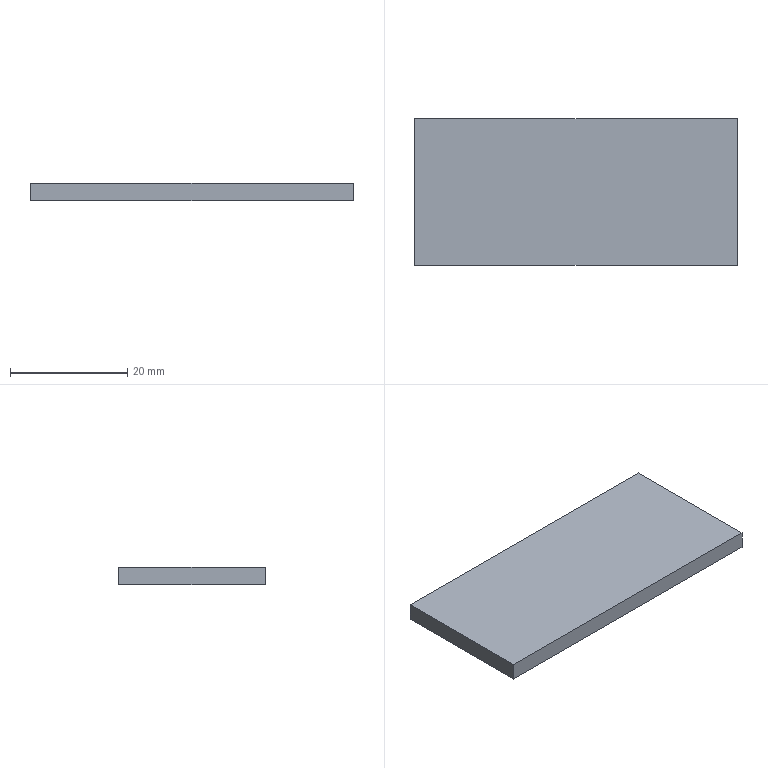Part | STEP file | 7101204 | 1 solid | 6 faces | box 55 x 25 x 3 mm | volume 4125 mm3 | plane 6
STEP:
#1=CARTESIAN_POINT('',(0.,0.,0.));
#2=DIRECTION('',(0.,0.,1.));
#3=DIRECTION('',(1.,0.,0.));
#4=AXIS2_PLACEMENT_3D('',#1,#2,#3);
#5=CARTESIAN_POINT('',(-56.43,-3.671,0.));
#6=VERTEX_POINT('',#5);
#7=CARTESIAN_POINT('',(-56.43,-28.671,0.));
#8=VERTEX_POINT('',#7);
#9=CARTESIAN_POINT('',(-56.43,-3.671,0.));
#10=DIRECTION('',(0.,-1.,0.));
#11=VECTOR('',#10,1.);
#12=LINE('',#9,#11);
#13=CARTESIAN_POINT('',(-56.43,-3.671,3.));
#14=DIRECTION('',(1.,0.,0.));
#15=DIRECTION('',(0.,1.,0.));
#16=AXIS2_PLACEMENT_3D('',#13,#14,#15);
#17=PLANE('',#16);
#18=CARTESIAN_POINT('',(0.,-3.));
#19=DIRECTION('',(-1.,0.));
#20=VECTOR('',#19,1.);
#21=LINE('',#18,#20);
#22=(GEOMETRIC_REPRESENTATION_CONTEXT(2)PARAMETRIC_REPRESENTATION_CONTEXT()REPRESENTATION_CONTEXT('',''));
#23=DEFINITIONAL_REPRESENTATION('',(#21),#22);
#24=PCURVE('',#17,#23);
#25=CARTESIAN_POINT('',(-56.43,-28.671,0.));
#26=DIRECTION('',(0.,0.,1.));
#27=DIRECTION('',(1.,0.,0.));
#28=AXIS2_PLACEMENT_3D('',#25,#26,#27);
#29=PLANE('',#28);
#30=CARTESIAN_POINT('',(0.,25.));
#31=DIRECTION('',(0.,-1.));
#32=VECTOR('',#31,1.);
#33=LINE('',#30,#32);
#34=(GEOMETRIC_REPRESENTATION_CONTEXT(2)PARAMETRIC_REPRESENTATION_CONTEXT()REPRESENTATION_CONTEXT('',''));
#35=DEFINITIONAL_REPRESENTATION('',(#33),#34);
#36=PCURVE('',#29,#35);
#37=SURFACE_CURVE('',#12,(#24,#36),.PCURVE_S1.);
#38=EDGE_CURVE('',#6,#8,#37,.T.);
#39=ORIENTED_EDGE('',*,*,#38,.T.);
#40=CARTESIAN_POINT('',(-56.43,-28.671,3.));
#41=VERTEX_POINT('',#40);
#42=CARTESIAN_POINT('',(-56.43,-28.671,3.));
#43=DIRECTION('',(0.,0.,-1.));
#44=VECTOR('',#43,1.);
#45=LINE('',#42,#44);
#46=CARTESIAN_POINT('',(-25.,0.));
#47=DIRECTION('',(0.,-1.));
#48=VECTOR('',#47,1.);
#49=LINE('',#46,#48);
#50=(GEOMETRIC_REPRESENTATION_CONTEXT(2)PARAMETRIC_REPRESENTATION_CONTEXT()REPRESENTATION_CONTEXT('',''));
#51=DEFINITIONAL_REPRESENTATION('',(#49),#50);
#52=PCURVE('',#17,#51);
#53=CARTESIAN_POINT('',(-56.43,-28.671,3.));
#54=DIRECTION('',(0.,1.,0.));
#55=DIRECTION('',(0.,0.,1.));
#56=AXIS2_PLACEMENT_3D('',#53,#54,#55);
#57=PLANE('',#56);
#58=CARTESIAN_POINT('',(0.,0.));
#59=DIRECTION('',(-1.,0.));
#60=VECTOR('',#59,1.);
#61=LINE('',#58,#60);
#62=(GEOMETRIC_REPRESENTATION_CONTEXT(2)PARAMETRIC_REPRESENTATION_CONTEXT()REPRESENTATION_CONTEXT('',''));
#63=DEFINITIONAL_REPRESENTATION('',(#61),#62);
#64=PCURVE('',#57,#63);
#65=SURFACE_CURVE('',#45,(#52,#64),.PCURVE_S1.);
#66=EDGE_CURVE('',#41,#8,#65,.T.);
#67=ORIENTED_EDGE('',*,*,#66,.F.);
#68=CARTESIAN_POINT('',(-56.43,-3.671,3.));
#69=VERTEX_POINT('',#68);
#70=CARTESIAN_POINT('',(-56.43,-3.671,3.));
#71=DIRECTION('',(0.,-1.,0.));
#72=VECTOR('',#71,1.);
#73=LINE('',#70,#72);
#74=CARTESIAN_POINT('',(0.,0.));
#75=DIRECTION('',(-1.,0.));
#76=VECTOR('',#75,1.);
#77=LINE('',#74,#76);
#78=(GEOMETRIC_REPRESENTATION_CONTEXT(2)PARAMETRIC_REPRESENTATION_CONTEXT()REPRESENTATION_CONTEXT('',''));
#79=DEFINITIONAL_REPRESENTATION('',(#77),#78);
#80=PCURVE('',#17,#79);
#81=CARTESIAN_POINT('',(-56.43,-28.671,3.));
#82=DIRECTION('',(0.,0.,1.));
#83=DIRECTION('',(1.,0.,0.));
#84=AXIS2_PLACEMENT_3D('',#81,#82,#83);
#85=PLANE('',#84);
#86=CARTESIAN_POINT('',(0.,25.));
#87=DIRECTION('',(0.,-1.));
#88=VECTOR('',#87,1.);
#89=LINE('',#86,#88);
#90=(GEOMETRIC_REPRESENTATION_CONTEXT(2)PARAMETRIC_REPRESENTATION_CONTEXT()REPRESENTATION_CONTEXT('',''));
#91=DEFINITIONAL_REPRESENTATION('',(#89),#90);
#92=PCURVE('',#85,#91);
#93=SURFACE_CURVE('',#73,(#80,#92),.PCURVE_S1.);
#94=EDGE_CURVE('',#69,#41,#93,.T.);
#95=ORIENTED_EDGE('',*,*,#94,.F.);
#96=CARTESIAN_POINT('',(-56.43,-3.671,3.));
#97=DIRECTION('',(0.,0.,-1.));
#98=VECTOR('',#97,1.);
#99=LINE('',#96,#98);
#100=CARTESIAN_POINT('',(0.,0.));
#101=DIRECTION('',(0.,-1.));
#102=VECTOR('',#101,1.);
#103=LINE('',#100,#102);
#104=(GEOMETRIC_REPRESENTATION_CONTEXT(2)PARAMETRIC_REPRESENTATION_CONTEXT()REPRESENTATION_CONTEXT('',''));
#105=DEFINITIONAL_REPRESENTATION('',(#103),#104);
#106=PCURVE('',#17,#105);
#107=CARTESIAN_POINT('',(-56.43,-3.671,3.));
#108=DIRECTION('',(0.,-1.,0.));
#109=DIRECTION('',(0.,0.,-1.));
#110=AXIS2_PLACEMENT_3D('',#107,#108,#109);
#111=PLANE('',#110);
#112=CARTESIAN_POINT('',(0.,0.));
#113=DIRECTION('',(1.,0.));
#114=VECTOR('',#113,1.);
#115=LINE('',#112,#114);
#116=(GEOMETRIC_REPRESENTATION_CONTEXT(2)PARAMETRIC_REPRESENTATION_CONTEXT()REPRESENTATION_CONTEXT('',''));
#117=DEFINITIONAL_REPRESENTATION('',(#115),#116);
#118=PCURVE('',#111,#117);
#119=SURFACE_CURVE('',#99,(#106,#118),.PCURVE_S1.);
#120=EDGE_CURVE('',#69,#6,#119,.T.);
#121=ORIENTED_EDGE('',*,*,#120,.T.);
#122=EDGE_LOOP('',(#39,#67,#95,#121));
#123=FACE_BOUND('',#122,.T.);
#124=ADVANCED_FACE('',(#123),#17,.F.);
#125=CARTESIAN_POINT('',(-1.43,-28.671,0.));
#126=VERTEX_POINT('',#125);
#127=CARTESIAN_POINT('',(-56.43,-28.671,0.));
#128=DIRECTION('',(1.,0.,0.));
#129=VECTOR('',#128,1.);
#130=LINE('',#127,#129);
#131=CARTESIAN_POINT('',(-3.,0.));
#132=DIRECTION('',(0.,1.));
#133=VECTOR('',#132,1.);
#134=LINE('',#131,#133);
#135=(GEOMETRIC_REPRESENTATION_CONTEXT(2)PARAMETRIC_REPRESENTATION_CONTEXT()REPRESENTATION_CONTEXT('',''));
#136=DEFINITIONAL_REPRESENTATION('',(#134),#135);
#137=PCURVE('',#57,#136);
#138=CARTESIAN_POINT('',(0.,0.));
#139=DIRECTION('',(1.,0.));
#140=VECTOR('',#139,1.);
#141=LINE('',#138,#140);
#142=(GEOMETRIC_REPRESENTATION_CONTEXT(2)PARAMETRIC_REPRESENTATION_CONTEXT()REPRESENTATION_CONTEXT('',''));
#143=DEFINITIONAL_REPRESENTATION('',(#141),#142);
#144=PCURVE('',#29,#143);
#145=SURFACE_CURVE('',#130,(#137,#144),.PCURVE_S1.);
#146=EDGE_CURVE('',#8,#126,#145,.T.);
#147=ORIENTED_EDGE('',*,*,#146,.T.);
#148=CARTESIAN_POINT('',(-1.43,-28.671,3.));
#149=VERTEX_POINT('',#148);
#150=CARTESIAN_POINT('',(-1.43,-28.671,3.));
#151=DIRECTION('',(0.,0.,-1.));
#152=VECTOR('',#151,1.);
#153=LINE('',#150,#152);
#154=CARTESIAN_POINT('',(0.,55.));
#155=DIRECTION('',(-1.,0.));
#156=VECTOR('',#155,1.);
#157=LINE('',#154,#156);
#158=(GEOMETRIC_REPRESENTATION_CONTEXT(2)PARAMETRIC_REPRESENTATION_CONTEXT()REPRESENTATION_CONTEXT('',''));
#159=DEFINITIONAL_REPRESENTATION('',(#157),#158);
#160=PCURVE('',#57,#159);
#161=CARTESIAN_POINT('',(-1.43,-3.671,3.));
#162=DIRECTION('',(-1.,0.,0.));
#163=DIRECTION('',(0.,0.,1.));
#164=AXIS2_PLACEMENT_3D('',#161,#162,#163);
#165=PLANE('',#164);
#166=CARTESIAN_POINT('',(0.,-25.));
#167=DIRECTION('',(-1.,0.));
#168=VECTOR('',#167,1.);
#169=LINE('',#166,#168);
#170=(GEOMETRIC_REPRESENTATION_CONTEXT(2)PARAMETRIC_REPRESENTATION_CONTEXT()REPRESENTATION_CONTEXT('',''));
#171=DEFINITIONAL_REPRESENTATION('',(#169),#170);
#172=PCURVE('',#165,#171);
#173=SURFACE_CURVE('',#153,(#160,#172),.PCURVE_S1.);
#174=EDGE_CURVE('',#149,#126,#173,.T.);
#175=ORIENTED_EDGE('',*,*,#174,.F.);
#176=CARTESIAN_POINT('',(-56.43,-28.671,3.));
#177=DIRECTION('',(1.,0.,0.));
#178=VECTOR('',#177,1.);
#179=LINE('',#176,#178);
#180=CARTESIAN_POINT('',(0.,0.));
#181=DIRECTION('',(0.,1.));
#182=VECTOR('',#181,1.);
#183=LINE('',#180,#182);
#184=(GEOMETRIC_REPRESENTATION_CONTEXT(2)PARAMETRIC_REPRESENTATION_CONTEXT()REPRESENTATION_CONTEXT('',''));
#185=DEFINITIONAL_REPRESENTATION('',(#183),#184);
#186=PCURVE('',#57,#185);
#187=CARTESIAN_POINT('',(0.,0.));
#188=DIRECTION('',(1.,0.));
#189=VECTOR('',#188,1.);
#190=LINE('',#187,#189);
#191=(GEOMETRIC_REPRESENTATION_CONTEXT(2)PARAMETRIC_REPRESENTATION_CONTEXT()REPRESENTATION_CONTEXT('',''));
#192=DEFINITIONAL_REPRESENTATION('',(#190),#191);
#193=PCURVE('',#85,#192);
#194=SURFACE_CURVE('',#179,(#186,#193),.PCURVE_S1.);
#195=EDGE_CURVE('',#41,#149,#194,.T.);
#196=ORIENTED_EDGE('',*,*,#195,.F.);
#197=ORIENTED_EDGE('',*,*,#66,.T.);
#198=EDGE_LOOP('',(#147,#175,#196,#197));
#199=FACE_BOUND('',#198,.T.);
#200=ADVANCED_FACE('',(#199),#57,.F.);
#201=CARTESIAN_POINT('',(-1.43,-3.671,0.));
#202=VERTEX_POINT('',#201);
#203=CARTESIAN_POINT('',(-1.43,-3.671,0.));
#204=DIRECTION('',(0.,1.,0.));
#205=VECTOR('',#204,1.);
#206=LINE('',#203,#205);
#207=CARTESIAN_POINT('',(-3.,0.));
#208=DIRECTION('',(0.,1.));
#209=VECTOR('',#208,1.);
#210=LINE('',#207,#209);
#211=(GEOMETRIC_REPRESENTATION_CONTEXT(2)PARAMETRIC_REPRESENTATION_CONTEXT()REPRESENTATION_CONTEXT('',''));
#212=DEFINITIONAL_REPRESENTATION('',(#210),#211);
#213=PCURVE('',#165,#212);
#214=CARTESIAN_POINT('',(55.,25.));
#215=DIRECTION('',(0.,1.));
#216=VECTOR('',#215,1.);
#217=LINE('',#214,#216);
#218=(GEOMETRIC_REPRESENTATION_CONTEXT(2)PARAMETRIC_REPRESENTATION_CONTEXT()REPRESENTATION_CONTEXT('',''));
#219=DEFINITIONAL_REPRESENTATION('',(#217),#218);
#220=PCURVE('',#29,#219);
#221=SURFACE_CURVE('',#206,(#213,#220),.PCURVE_S1.);
#222=EDGE_CURVE('',#126,#202,#221,.T.);
#223=ORIENTED_EDGE('',*,*,#222,.T.);
#224=CARTESIAN_POINT('',(-1.43,-3.671,3.));
#225=VERTEX_POINT('',#224);
#226=CARTESIAN_POINT('',(-1.43,-3.671,3.));
#227=DIRECTION('',(0.,0.,-1.));
#228=VECTOR('',#227,1.);
#229=LINE('',#226,#228);
#230=CARTESIAN_POINT('',(0.,0.));
#231=DIRECTION('',(-1.,0.));
#232=VECTOR('',#231,1.);
#233=LINE('',#230,#232);
#234=(GEOMETRIC_REPRESENTATION_CONTEXT(2)PARAMETRIC_REPRESENTATION_CONTEXT()REPRESENTATION_CONTEXT('',''));
#235=DEFINITIONAL_REPRESENTATION('',(#233),#234);
#236=PCURVE('',#165,#235);
#237=CARTESIAN_POINT('',(0.,55.));
#238=DIRECTION('',(1.,0.));
#239=VECTOR('',#238,1.);
#240=LINE('',#237,#239);
#241=(GEOMETRIC_REPRESENTATION_CONTEXT(2)PARAMETRIC_REPRESENTATION_CONTEXT()REPRESENTATION_CONTEXT('',''));
#242=DEFINITIONAL_REPRESENTATION('',(#240),#241);
#243=PCURVE('',#111,#242);
#244=SURFACE_CURVE('',#229,(#236,#243),.PCURVE_S1.);
#245=EDGE_CURVE('',#225,#202,#244,.T.);
#246=ORIENTED_EDGE('',*,*,#245,.F.);
#247=CARTESIAN_POINT('',(-1.43,-3.671,3.));
#248=DIRECTION('',(0.,1.,0.));
#249=VECTOR('',#248,1.);
#250=LINE('',#247,#249);
#251=CARTESIAN_POINT('',(0.,0.));
#252=DIRECTION('',(0.,1.));
#253=VECTOR('',#252,1.);
#254=LINE('',#251,#253);
#255=(GEOMETRIC_REPRESENTATION_CONTEXT(2)PARAMETRIC_REPRESENTATION_CONTEXT()REPRESENTATION_CONTEXT('',''));
#256=DEFINITIONAL_REPRESENTATION('',(#254),#255);
#257=PCURVE('',#165,#256);
#258=CARTESIAN_POINT('',(55.,25.));
#259=DIRECTION('',(0.,1.));
#260=VECTOR('',#259,1.);
#261=LINE('',#258,#260);
#262=(GEOMETRIC_REPRESENTATION_CONTEXT(2)PARAMETRIC_REPRESENTATION_CONTEXT()REPRESENTATION_CONTEXT('',''));
#263=DEFINITIONAL_REPRESENTATION('',(#261),#262);
#264=PCURVE('',#85,#263);
#265=SURFACE_CURVE('',#250,(#257,#264),.PCURVE_S1.);
#266=EDGE_CURVE('',#149,#225,#265,.T.);
#267=ORIENTED_EDGE('',*,*,#266,.F.);
#268=ORIENTED_EDGE('',*,*,#174,.T.);
#269=EDGE_LOOP('',(#223,#246,#267,#268));
#270=FACE_BOUND('',#269,.T.);
#271=ADVANCED_FACE('',(#270),#165,.F.);
#272=CARTESIAN_POINT('',(-56.43,-3.671,0.));
#273=DIRECTION('',(-1.,0.,0.));
#274=VECTOR('',#273,1.);
#275=LINE('',#272,#274);
#276=CARTESIAN_POINT('',(3.,0.));
#277=DIRECTION('',(0.,-1.));
#278=VECTOR('',#277,1.);
#279=LINE('',#276,#278);
#280=(GEOMETRIC_REPRESENTATION_CONTEXT(2)PARAMETRIC_REPRESENTATION_CONTEXT()REPRESENTATION_CONTEXT('',''));
#281=DEFINITIONAL_REPRESENTATION('',(#279),#280);
#282=PCURVE('',#111,#281);
#283=CARTESIAN_POINT('',(0.,25.));
#284=DIRECTION('',(-1.,0.));
#285=VECTOR('',#284,1.);
#286=LINE('',#283,#285);
#287=(GEOMETRIC_REPRESENTATION_CONTEXT(2)PARAMETRIC_REPRESENTATION_CONTEXT()REPRESENTATION_CONTEXT('',''));
#288=DEFINITIONAL_REPRESENTATION('',(#286),#287);
#289=PCURVE('',#29,#288);
#290=SURFACE_CURVE('',#275,(#282,#289),.PCURVE_S1.);
#291=EDGE_CURVE('',#202,#6,#290,.T.);
#292=ORIENTED_EDGE('',*,*,#291,.T.);
#293=ORIENTED_EDGE('',*,*,#120,.F.);
#294=CARTESIAN_POINT('',(-56.43,-3.671,3.));
#295=DIRECTION('',(-1.,0.,0.));
#296=VECTOR('',#295,1.);
#297=LINE('',#294,#296);
#298=CARTESIAN_POINT('',(0.,0.));
#299=DIRECTION('',(0.,-1.));
#300=VECTOR('',#299,1.);
#301=LINE('',#298,#300);
#302=(GEOMETRIC_REPRESENTATION_CONTEXT(2)PARAMETRIC_REPRESENTATION_CONTEXT()REPRESENTATION_CONTEXT('',''));
#303=DEFINITIONAL_REPRESENTATION('',(#301),#302);
#304=PCURVE('',#111,#303);
#305=CARTESIAN_POINT('',(0.,25.));
#306=DIRECTION('',(-1.,0.));
#307=VECTOR('',#306,1.);
#308=LINE('',#305,#307);
#309=(GEOMETRIC_REPRESENTATION_CONTEXT(2)PARAMETRIC_REPRESENTATION_CONTEXT()REPRESENTATION_CONTEXT('',''));
#310=DEFINITIONAL_REPRESENTATION('',(#308),#309);
#311=PCURVE('',#85,#310);
#312=SURFACE_CURVE('',#297,(#304,#311),.PCURVE_S1.);
#313=EDGE_CURVE('',#225,#69,#312,.T.);
#314=ORIENTED_EDGE('',*,*,#313,.F.);
#315=ORIENTED_EDGE('',*,*,#245,.T.);
#316=EDGE_LOOP('',(#292,#293,#314,#315));
#317=FACE_BOUND('',#316,.T.);
#318=ADVANCED_FACE('',(#317),#111,.F.);
#319=ORIENTED_EDGE('',*,*,#94,.T.);
#320=ORIENTED_EDGE('',*,*,#195,.T.);
#321=ORIENTED_EDGE('',*,*,#266,.T.);
#322=ORIENTED_EDGE('',*,*,#313,.T.);
#323=EDGE_LOOP('',(#319,#320,#321,#322));
#324=FACE_BOUND('',#323,.T.);
#325=ADVANCED_FACE('',(#324),#85,.T.);
#326=ORIENTED_EDGE('',*,*,#38,.F.);
#327=ORIENTED_EDGE('',*,*,#291,.F.);
#328=ORIENTED_EDGE('',*,*,#222,.F.);
#329=ORIENTED_EDGE('',*,*,#146,.F.);
#330=EDGE_LOOP('',(#326,#327,#328,#329));
#331=FACE_BOUND('',#330,.T.);
#332=ADVANCED_FACE('',(#331),#29,.F.);
#333=CLOSED_SHELL('',(#124,#200,#271,#318,#325,#332));
#334=MANIFOLD_SOLID_BREP('',#333);
#335=(LENGTH_UNIT()NAMED_UNIT(*)SI_UNIT(.MILLI.,.METRE.));
#336=UNCERTAINTY_MEASURE_WITH_UNIT(LENGTH_MEASURE(0.0000001),#335,'','');
#337=(NAMED_UNIT(*)PLANE_ANGLE_UNIT()SI_UNIT($,.RADIAN.));
#338=(NAMED_UNIT(*)SI_UNIT($,.STERADIAN.)SOLID_ANGLE_UNIT());
#339=(GEOMETRIC_REPRESENTATION_CONTEXT(3)GLOBAL_UNCERTAINTY_ASSIGNED_CONTEXT((#336))GLOBAL_UNIT_ASSIGNED_CONTEXT((#335,#337,#338))REPRESENTATION_CONTEXT('',''));
#340=ADVANCED_BREP_SHAPE_REPRESENTATION('',(#4,#334),#339);